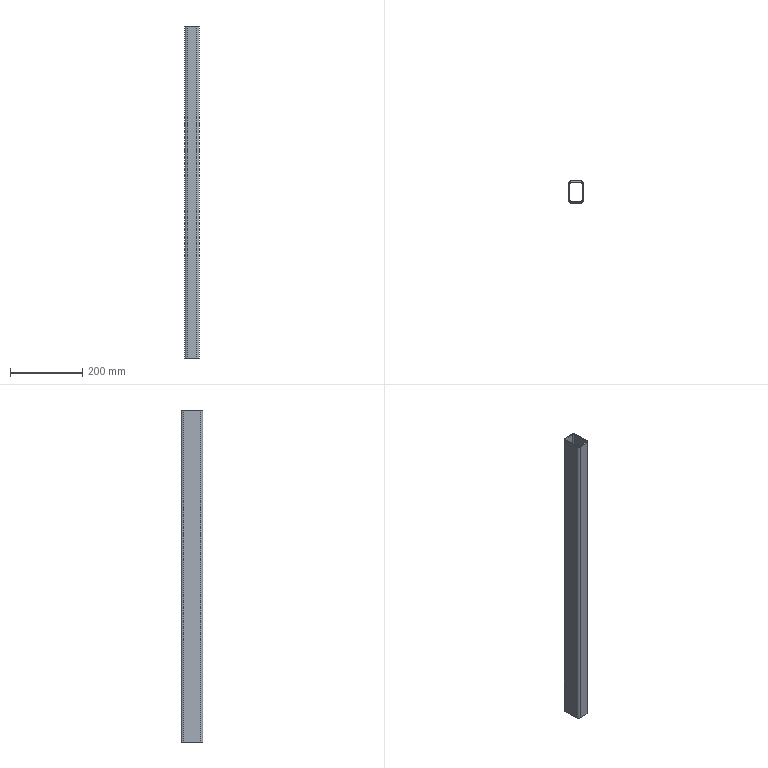Part | STEP file | Profile 4060920 | 1 solid | 18 faces | box 40 x 60 x 920 mm | volume 526856 mm3 | plane 10 | cylinder 8 | commonest cylinder face diameters 6.4 x4 12.8 x4
STEP:
#1=CARTESIAN_POINT('',(40.,6.4,-600.));
#2=VERTEX_POINT('',#1);
#3=CARTESIAN_POINT('',(40.,6.4,320.));
#4=VERTEX_POINT('',#3);
#5=CARTESIAN_POINT('',(40.,6.4,600.));
#6=DIRECTION('',(0.,0.,1.));
#7=VECTOR('',#6,1000.);
#8=LINE('',#5,#7);
#9=EDGE_CURVE('',#2,#4,#8,.T.);
#10=ORIENTED_EDGE('',*,*,#9,.F.);
#11=CARTESIAN_POINT('',(40.,53.6,-600.));
#12=VERTEX_POINT('',#11);
#13=CARTESIAN_POINT('',(40.,53.6,-600.));
#14=DIRECTION('',(0.,-1.,0.));
#15=VECTOR('',#14,1000.);
#16=LINE('',#13,#15);
#17=EDGE_CURVE('',#12,#2,#16,.T.);
#18=ORIENTED_EDGE('',*,*,#17,.F.);
#19=CARTESIAN_POINT('',(40.,53.6,320.));
#20=VERTEX_POINT('',#19);
#21=CARTESIAN_POINT('',(40.,53.6,600.));
#22=DIRECTION('',(0.,0.,-1.));
#23=VECTOR('',#22,1000.);
#24=LINE('',#21,#23);
#25=EDGE_CURVE('',#20,#12,#24,.T.);
#26=ORIENTED_EDGE('',*,*,#25,.F.);
#27=CARTESIAN_POINT('',(40.,53.6,320.));
#28=DIRECTION('',(0.,1.,0.));
#29=VECTOR('',#28,1000.);
#30=LINE('',#27,#29);
#31=EDGE_CURVE('',#4,#20,#30,.T.);
#32=ORIENTED_EDGE('',*,*,#31,.F.);
#33=EDGE_LOOP('',(#10,#18,#26,#32));
#34=FACE_OUTER_BOUND('',#33,.T.);
#35=CARTESIAN_POINT('',(40.,53.6,600.));
#36=DIRECTION('',(-1.,0.,0.));
#37=DIRECTION('',(0.,0.,1.));
#38=AXIS2_PLACEMENT_3D('',#35,#36,#37);
#39=PLANE('',#38);
#40=ADVANCED_FACE('',(#34),#39,.F.);
#41=CARTESIAN_POINT('',(0.,6.4,320.));
#42=VERTEX_POINT('',#41);
#43=CARTESIAN_POINT('',(6.4,0.,320.));
#44=VERTEX_POINT('',#43);
#45=CARTESIAN_POINT('',(6.4,6.4,320.));
#46=DIRECTION('',(0.,0.,1.));
#47=DIRECTION('',(-1.,0.,0.));
#48=AXIS2_PLACEMENT_3D('',#45,#46,#47);
#49=CIRCLE('',#48,6.4);
#50=EDGE_CURVE('',#42,#44,#49,.T.);
#51=ORIENTED_EDGE('',*,*,#50,.T.);
#52=CARTESIAN_POINT('',(33.6,0.,320.));
#53=VERTEX_POINT('',#52);
#54=CARTESIAN_POINT('',(33.6,0.,320.));
#55=DIRECTION('',(1.,0.,0.));
#56=VECTOR('',#55,1000.);
#57=LINE('',#54,#56);
#58=EDGE_CURVE('',#44,#53,#57,.T.);
#59=ORIENTED_EDGE('',*,*,#58,.T.);
#60=CARTESIAN_POINT('',(33.6,6.4,320.));
#61=DIRECTION('',(0.,0.,1.));
#62=DIRECTION('',(-1.,0.,0.));
#63=AXIS2_PLACEMENT_3D('',#60,#61,#62);
#64=CIRCLE('',#63,6.4);
#65=EDGE_CURVE('',#53,#4,#64,.T.);
#66=ORIENTED_EDGE('',*,*,#65,.T.);
#67=ORIENTED_EDGE('',*,*,#31,.T.);
#68=CARTESIAN_POINT('',(33.6,60.,320.));
#69=VERTEX_POINT('',#68);
#70=CARTESIAN_POINT('',(33.6,53.6,320.));
#71=DIRECTION('',(0.,0.,1.));
#72=DIRECTION('',(-1.,0.,0.));
#73=AXIS2_PLACEMENT_3D('',#70,#71,#72);
#74=CIRCLE('',#73,6.4);
#75=EDGE_CURVE('',#20,#69,#74,.T.);
#76=ORIENTED_EDGE('',*,*,#75,.T.);
#77=CARTESIAN_POINT('',(6.4,60.,320.));
#78=VERTEX_POINT('',#77);
#79=CARTESIAN_POINT('',(33.6,60.,320.));
#80=DIRECTION('',(-1.,0.,0.));
#81=VECTOR('',#80,1000.);
#82=LINE('',#79,#81);
#83=EDGE_CURVE('',#69,#78,#82,.T.);
#84=ORIENTED_EDGE('',*,*,#83,.T.);
#85=CARTESIAN_POINT('',(0.,53.6,320.));
#86=VERTEX_POINT('',#85);
#87=CARTESIAN_POINT('',(6.4,53.6,320.));
#88=DIRECTION('',(0.,0.,1.));
#89=DIRECTION('',(-1.,0.,0.));
#90=AXIS2_PLACEMENT_3D('',#87,#88,#89);
#91=CIRCLE('',#90,6.4);
#92=EDGE_CURVE('',#78,#86,#91,.T.);
#93=ORIENTED_EDGE('',*,*,#92,.T.);
#94=CARTESIAN_POINT('',(0.,6.4,320.));
#95=DIRECTION('',(0.,-1.,0.));
#96=VECTOR('',#95,1000.);
#97=LINE('',#94,#96);
#98=EDGE_CURVE('',#86,#42,#97,.T.);
#99=ORIENTED_EDGE('',*,*,#98,.T.);
#100=EDGE_LOOP('',(#51,#59,#66,#67,#76,#84,#93,#99));
#101=FACE_OUTER_BOUND('',#100,.T.);
#102=CARTESIAN_POINT('',(36.8,53.6,320.));
#103=VERTEX_POINT('',#102);
#104=CARTESIAN_POINT('',(36.8,6.4,320.));
#105=VERTEX_POINT('',#104);
#106=CARTESIAN_POINT('',(36.8,6.4,320.));
#107=DIRECTION('',(0.,-1.,0.));
#108=VECTOR('',#107,1000.);
#109=LINE('',#106,#108);
#110=EDGE_CURVE('',#103,#105,#109,.T.);
#111=ORIENTED_EDGE('',*,*,#110,.T.);
#112=CARTESIAN_POINT('',(33.6,3.2,320.));
#113=VERTEX_POINT('',#112);
#114=CARTESIAN_POINT('',(33.6,6.4,320.));
#115=DIRECTION('',(0.,0.,-1.));
#116=DIRECTION('',(-1.,0.,0.));
#117=AXIS2_PLACEMENT_3D('',#114,#115,#116);
#118=CIRCLE('',#117,3.2);
#119=EDGE_CURVE('',#105,#113,#118,.T.);
#120=ORIENTED_EDGE('',*,*,#119,.T.);
#121=CARTESIAN_POINT('',(6.4,3.2,320.));
#122=VERTEX_POINT('',#121);
#123=CARTESIAN_POINT('',(33.6,3.2,320.));
#124=DIRECTION('',(-1.,0.,0.));
#125=VECTOR('',#124,1000.);
#126=LINE('',#123,#125);
#127=EDGE_CURVE('',#113,#122,#126,.T.);
#128=ORIENTED_EDGE('',*,*,#127,.T.);
#129=CARTESIAN_POINT('',(3.2,6.4,320.));
#130=VERTEX_POINT('',#129);
#131=CARTESIAN_POINT('',(6.4,6.4,320.));
#132=DIRECTION('',(0.,0.,-1.));
#133=DIRECTION('',(-1.,0.,0.));
#134=AXIS2_PLACEMENT_3D('',#131,#132,#133);
#135=CIRCLE('',#134,3.2);
#136=EDGE_CURVE('',#122,#130,#135,.T.);
#137=ORIENTED_EDGE('',*,*,#136,.T.);
#138=CARTESIAN_POINT('',(3.2,53.6,320.));
#139=VERTEX_POINT('',#138);
#140=CARTESIAN_POINT('',(3.2,6.4,320.));
#141=DIRECTION('',(0.,1.,0.));
#142=VECTOR('',#141,1000.);
#143=LINE('',#140,#142);
#144=EDGE_CURVE('',#130,#139,#143,.T.);
#145=ORIENTED_EDGE('',*,*,#144,.T.);
#146=CARTESIAN_POINT('',(6.4,56.8,320.));
#147=VERTEX_POINT('',#146);
#148=CARTESIAN_POINT('',(6.4,53.6,320.));
#149=DIRECTION('',(0.,0.,-1.));
#150=DIRECTION('',(-1.,0.,0.));
#151=AXIS2_PLACEMENT_3D('',#148,#149,#150);
#152=CIRCLE('',#151,3.2);
#153=EDGE_CURVE('',#139,#147,#152,.T.);
#154=ORIENTED_EDGE('',*,*,#153,.T.);
#155=CARTESIAN_POINT('',(33.6,56.8,320.));
#156=VERTEX_POINT('',#155);
#157=CARTESIAN_POINT('',(33.6,56.8,320.));
#158=DIRECTION('',(1.,0.,0.));
#159=VECTOR('',#158,1000.);
#160=LINE('',#157,#159);
#161=EDGE_CURVE('',#147,#156,#160,.T.);
#162=ORIENTED_EDGE('',*,*,#161,.T.);
#163=CARTESIAN_POINT('',(33.6,53.6,320.));
#164=DIRECTION('',(0.,0.,-1.));
#165=DIRECTION('',(-1.,0.,0.));
#166=AXIS2_PLACEMENT_3D('',#163,#164,#165);
#167=CIRCLE('',#166,3.2);
#168=EDGE_CURVE('',#156,#103,#167,.T.);
#169=ORIENTED_EDGE('',*,*,#168,.T.);
#170=EDGE_LOOP('',(#111,#120,#128,#137,#145,#154,#162,#169));
#171=FACE_BOUND('',#170,.T.);
#172=CARTESIAN_POINT('',(33.6,6.4,320.));
#173=DIRECTION('',(0.,0.,1.));
#174=DIRECTION('',(1.,0.,0.));
#175=AXIS2_PLACEMENT_3D('',#172,#173,#174);
#176=PLANE('',#175);
#177=ADVANCED_FACE('',(#101,#171),#176,.T.);
#178=CARTESIAN_POINT('',(33.6,0.,-600.));
#179=VERTEX_POINT('',#178);
#180=CARTESIAN_POINT('',(33.6,0.,600.));
#181=DIRECTION('',(0.,0.,-1.));
#182=VECTOR('',#181,1000.);
#183=LINE('',#180,#182);
#184=EDGE_CURVE('',#53,#179,#183,.T.);
#185=ORIENTED_EDGE('',*,*,#184,.T.);
#186=CARTESIAN_POINT('',(33.6,6.4,-600.));
#187=DIRECTION('',(0.,0.,1.));
#188=DIRECTION('',(-1.,0.,0.));
#189=AXIS2_PLACEMENT_3D('',#186,#187,#188);
#190=CIRCLE('',#189,6.4);
#191=EDGE_CURVE('',#179,#2,#190,.T.);
#192=ORIENTED_EDGE('',*,*,#191,.T.);
#193=ORIENTED_EDGE('',*,*,#9,.T.);
#194=ORIENTED_EDGE('',*,*,#65,.F.);
#195=EDGE_LOOP('',(#185,#192,#193,#194));
#196=FACE_OUTER_BOUND('',#195,.T.);
#197=CARTESIAN_POINT('',(33.6,6.4,600.));
#198=DIRECTION('',(0.,0.,-1.));
#199=DIRECTION('',(-1.,0.,0.));
#200=AXIS2_PLACEMENT_3D('',#197,#198,#199);
#201=CYLINDRICAL_SURFACE('',#200,6.4);
#202=ADVANCED_FACE('',(#196),#201,.T.);
#203=ORIENTED_EDGE('',*,*,#191,.F.);
#204=CARTESIAN_POINT('',(6.4,0.,-600.));
#205=VERTEX_POINT('',#204);
#206=CARTESIAN_POINT('',(33.6,0.,-600.));
#207=DIRECTION('',(1.,0.,0.));
#208=VECTOR('',#207,1000.);
#209=LINE('',#206,#208);
#210=EDGE_CURVE('',#205,#179,#209,.T.);
#211=ORIENTED_EDGE('',*,*,#210,.F.);
#212=CARTESIAN_POINT('',(0.,6.4,-600.));
#213=VERTEX_POINT('',#212);
#214=CARTESIAN_POINT('',(6.4,6.4,-600.));
#215=DIRECTION('',(0.,0.,1.));
#216=DIRECTION('',(-1.,0.,0.));
#217=AXIS2_PLACEMENT_3D('',#214,#215,#216);
#218=CIRCLE('',#217,6.4);
#219=EDGE_CURVE('',#213,#205,#218,.T.);
#220=ORIENTED_EDGE('',*,*,#219,.F.);
#221=CARTESIAN_POINT('',(0.,53.6,-600.));
#222=VERTEX_POINT('',#221);
#223=CARTESIAN_POINT('',(0.,53.6,-600.));
#224=DIRECTION('',(0.,-1.,0.));
#225=VECTOR('',#224,1000.);
#226=LINE('',#223,#225);
#227=EDGE_CURVE('',#222,#213,#226,.T.);
#228=ORIENTED_EDGE('',*,*,#227,.F.);
#229=CARTESIAN_POINT('',(6.4,60.,-600.));
#230=VERTEX_POINT('',#229);
#231=CARTESIAN_POINT('',(6.4,53.6,-600.));
#232=DIRECTION('',(0.,0.,1.));
#233=DIRECTION('',(-1.,0.,0.));
#234=AXIS2_PLACEMENT_3D('',#231,#232,#233);
#235=CIRCLE('',#234,6.4);
#236=EDGE_CURVE('',#230,#222,#235,.T.);
#237=ORIENTED_EDGE('',*,*,#236,.F.);
#238=CARTESIAN_POINT('',(33.6,60.,-600.));
#239=VERTEX_POINT('',#238);
#240=CARTESIAN_POINT('',(33.6,60.,-600.));
#241=DIRECTION('',(-1.,0.,0.));
#242=VECTOR('',#241,1000.);
#243=LINE('',#240,#242);
#244=EDGE_CURVE('',#239,#230,#243,.T.);
#245=ORIENTED_EDGE('',*,*,#244,.F.);
#246=CARTESIAN_POINT('',(33.6,53.6,-600.));
#247=DIRECTION('',(0.,0.,1.));
#248=DIRECTION('',(-1.,0.,0.));
#249=AXIS2_PLACEMENT_3D('',#246,#247,#248);
#250=CIRCLE('',#249,6.4);
#251=EDGE_CURVE('',#12,#239,#250,.T.);
#252=ORIENTED_EDGE('',*,*,#251,.F.);
#253=ORIENTED_EDGE('',*,*,#17,.T.);
#254=EDGE_LOOP('',(#203,#211,#220,#228,#237,#245,#252,#253));
#255=FACE_OUTER_BOUND('',#254,.T.);
#256=CARTESIAN_POINT('',(6.4,3.2,-600.));
#257=VERTEX_POINT('',#256);
#258=CARTESIAN_POINT('',(3.2,6.4,-600.));
#259=VERTEX_POINT('',#258);
#260=CARTESIAN_POINT('',(6.4,6.4,-600.));
#261=DIRECTION('',(0.,0.,-1.));
#262=DIRECTION('',(-1.,0.,0.));
#263=AXIS2_PLACEMENT_3D('',#260,#261,#262);
#264=CIRCLE('',#263,3.2);
#265=EDGE_CURVE('',#257,#259,#264,.T.);
#266=ORIENTED_EDGE('',*,*,#265,.F.);
#267=CARTESIAN_POINT('',(33.6,3.2,-600.));
#268=VERTEX_POINT('',#267);
#269=CARTESIAN_POINT('',(33.6,3.2,-600.));
#270=DIRECTION('',(-1.,0.,0.));
#271=VECTOR('',#270,1000.);
#272=LINE('',#269,#271);
#273=EDGE_CURVE('',#268,#257,#272,.T.);
#274=ORIENTED_EDGE('',*,*,#273,.F.);
#275=CARTESIAN_POINT('',(36.8,6.4,-600.));
#276=VERTEX_POINT('',#275);
#277=CARTESIAN_POINT('',(33.6,6.4,-600.));
#278=DIRECTION('',(0.,0.,-1.));
#279=DIRECTION('',(-1.,0.,0.));
#280=AXIS2_PLACEMENT_3D('',#277,#278,#279);
#281=CIRCLE('',#280,3.2);
#282=EDGE_CURVE('',#276,#268,#281,.T.);
#283=ORIENTED_EDGE('',*,*,#282,.F.);
#284=CARTESIAN_POINT('',(36.8,53.6,-600.));
#285=VERTEX_POINT('',#284);
#286=CARTESIAN_POINT('',(36.8,53.6,-600.));
#287=DIRECTION('',(0.,-1.,0.));
#288=VECTOR('',#287,1000.);
#289=LINE('',#286,#288);
#290=EDGE_CURVE('',#285,#276,#289,.T.);
#291=ORIENTED_EDGE('',*,*,#290,.F.);
#292=CARTESIAN_POINT('',(33.6,56.8,-600.));
#293=VERTEX_POINT('',#292);
#294=CARTESIAN_POINT('',(33.6,53.6,-600.));
#295=DIRECTION('',(0.,0.,-1.));
#296=DIRECTION('',(-1.,0.,0.));
#297=AXIS2_PLACEMENT_3D('',#294,#295,#296);
#298=CIRCLE('',#297,3.2);
#299=EDGE_CURVE('',#293,#285,#298,.T.);
#300=ORIENTED_EDGE('',*,*,#299,.F.);
#301=CARTESIAN_POINT('',(6.4,56.8,-600.));
#302=VERTEX_POINT('',#301);
#303=CARTESIAN_POINT('',(33.6,56.8,-600.));
#304=DIRECTION('',(1.,0.,0.));
#305=VECTOR('',#304,1000.);
#306=LINE('',#303,#305);
#307=EDGE_CURVE('',#302,#293,#306,.T.);
#308=ORIENTED_EDGE('',*,*,#307,.F.);
#309=CARTESIAN_POINT('',(3.2,53.6,-600.));
#310=VERTEX_POINT('',#309);
#311=CARTESIAN_POINT('',(6.4,53.6,-600.));
#312=DIRECTION('',(0.,0.,-1.));
#313=DIRECTION('',(-1.,0.,0.));
#314=AXIS2_PLACEMENT_3D('',#311,#312,#313);
#315=CIRCLE('',#314,3.2);
#316=EDGE_CURVE('',#310,#302,#315,.T.);
#317=ORIENTED_EDGE('',*,*,#316,.F.);
#318=CARTESIAN_POINT('',(3.2,53.6,-600.));
#319=DIRECTION('',(0.,1.,0.));
#320=VECTOR('',#319,1000.);
#321=LINE('',#318,#320);
#322=EDGE_CURVE('',#259,#310,#321,.T.);
#323=ORIENTED_EDGE('',*,*,#322,.F.);
#324=EDGE_LOOP('',(#266,#274,#283,#291,#300,#308,#317,#323));
#325=FACE_BOUND('',#324,.T.);
#326=CARTESIAN_POINT('',(33.6,53.6,-600.));
#327=DIRECTION('',(0.,0.,1.));
#328=DIRECTION('',(1.,0.,0.));
#329=AXIS2_PLACEMENT_3D('',#326,#327,#328);
#330=PLANE('',#329);
#331=ADVANCED_FACE('',(#255,#325),#330,.F.);
#332=ORIENTED_EDGE('',*,*,#25,.T.);
#333=ORIENTED_EDGE('',*,*,#251,.T.);
#334=CARTESIAN_POINT('',(33.6,60.,600.));
#335=DIRECTION('',(0.,0.,1.));
#336=VECTOR('',#335,1000.);
#337=LINE('',#334,#336);
#338=EDGE_CURVE('',#239,#69,#337,.T.);
#339=ORIENTED_EDGE('',*,*,#338,.T.);
#340=ORIENTED_EDGE('',*,*,#75,.F.);
#341=EDGE_LOOP('',(#332,#333,#339,#340));
#342=FACE_OUTER_BOUND('',#341,.T.);
#343=CARTESIAN_POINT('',(33.6,53.6,600.));
#344=DIRECTION('',(0.,0.,-1.));
#345=DIRECTION('',(-1.,0.,0.));
#346=AXIS2_PLACEMENT_3D('',#343,#344,#345);
#347=CYLINDRICAL_SURFACE('',#346,6.4);
#348=ADVANCED_FACE('',(#342),#347,.T.);
#349=CARTESIAN_POINT('',(6.4,0.,600.));
#350=DIRECTION('',(0.,0.,1.));
#351=VECTOR('',#350,1000.);
#352=LINE('',#349,#351);
#353=EDGE_CURVE('',#205,#44,#352,.T.);
#354=ORIENTED_EDGE('',*,*,#353,.F.);
#355=ORIENTED_EDGE('',*,*,#210,.T.);
#356=ORIENTED_EDGE('',*,*,#184,.F.);
#357=ORIENTED_EDGE('',*,*,#58,.F.);
#358=EDGE_LOOP('',(#354,#355,#356,#357));
#359=FACE_OUTER_BOUND('',#358,.T.);
#360=CARTESIAN_POINT('',(6.4,0.,600.));
#361=DIRECTION('',(0.,1.,0.));
#362=DIRECTION('',(-1.,0.,0.));
#363=AXIS2_PLACEMENT_3D('',#360,#361,#362);
#364=PLANE('',#363);
#365=ADVANCED_FACE('',(#359),#364,.F.);
#366=CARTESIAN_POINT('',(0.,6.4,600.));
#367=DIRECTION('',(0.,0.,-1.));
#368=VECTOR('',#367,1000.);
#369=LINE('',#366,#368);
#370=EDGE_CURVE('',#42,#213,#369,.T.);
#371=ORIENTED_EDGE('',*,*,#370,.T.);
#372=ORIENTED_EDGE('',*,*,#219,.T.);
#373=ORIENTED_EDGE('',*,*,#353,.T.);
#374=ORIENTED_EDGE('',*,*,#50,.F.);
#375=EDGE_LOOP('',(#371,#372,#373,#374));
#376=FACE_OUTER_BOUND('',#375,.T.);
#377=CARTESIAN_POINT('',(6.4,6.4,600.));
#378=DIRECTION('',(0.,0.,-1.));
#379=DIRECTION('',(-1.,0.,0.));
#380=AXIS2_PLACEMENT_3D('',#377,#378,#379);
#381=CYLINDRICAL_SURFACE('',#380,6.4);
#382=ADVANCED_FACE('',(#376),#381,.T.);
#383=CARTESIAN_POINT('',(0.,53.6,600.));
#384=DIRECTION('',(0.,0.,1.));
#385=VECTOR('',#384,1000.);
#386=LINE('',#383,#385);
#387=EDGE_CURVE('',#222,#86,#386,.T.);
#388=ORIENTED_EDGE('',*,*,#387,.F.);
#389=ORIENTED_EDGE('',*,*,#227,.T.);
#390=ORIENTED_EDGE('',*,*,#370,.F.);
#391=ORIENTED_EDGE('',*,*,#98,.F.);
#392=EDGE_LOOP('',(#388,#389,#390,#391));
#393=FACE_OUTER_BOUND('',#392,.T.);
#394=CARTESIAN_POINT('',(0.,6.4,600.));
#395=DIRECTION('',(1.,0.,0.));
#396=DIRECTION('',(0.,1.,0.));
#397=AXIS2_PLACEMENT_3D('',#394,#395,#396);
#398=PLANE('',#397);
#399=ADVANCED_FACE('',(#393),#398,.F.);
#400=CARTESIAN_POINT('',(6.4,60.,600.));
#401=DIRECTION('',(0.,0.,-1.));
#402=VECTOR('',#401,1000.);
#403=LINE('',#400,#402);
#404=EDGE_CURVE('',#78,#230,#403,.T.);
#405=ORIENTED_EDGE('',*,*,#404,.T.);
#406=ORIENTED_EDGE('',*,*,#236,.T.);
#407=ORIENTED_EDGE('',*,*,#387,.T.);
#408=ORIENTED_EDGE('',*,*,#92,.F.);
#409=EDGE_LOOP('',(#405,#406,#407,#408));
#410=FACE_OUTER_BOUND('',#409,.T.);
#411=CARTESIAN_POINT('',(6.4,53.6,600.));
#412=DIRECTION('',(0.,0.,-1.));
#413=DIRECTION('',(-1.,0.,0.));
#414=AXIS2_PLACEMENT_3D('',#411,#412,#413);
#415=CYLINDRICAL_SURFACE('',#414,6.4);
#416=ADVANCED_FACE('',(#410),#415,.T.);
#417=ORIENTED_EDGE('',*,*,#338,.F.);
#418=ORIENTED_EDGE('',*,*,#244,.T.);
#419=ORIENTED_EDGE('',*,*,#404,.F.);
#420=ORIENTED_EDGE('',*,*,#83,.F.);
#421=EDGE_LOOP('',(#417,#418,#419,#420));
#422=FACE_OUTER_BOUND('',#421,.T.);
#423=CARTESIAN_POINT('',(33.6,60.,600.));
#424=DIRECTION('',(0.,-1.,0.));
#425=DIRECTION('',(0.,0.,-1.));
#426=AXIS2_PLACEMENT_3D('',#423,#424,#425);
#427=PLANE('',#426);
#428=ADVANCED_FACE('',(#422),#427,.F.);
#429=CARTESIAN_POINT('',(36.8,6.4,600.));
#430=DIRECTION('',(0.,0.,1.));
#431=VECTOR('',#430,1000.);
#432=LINE('',#429,#431);
#433=EDGE_CURVE('',#276,#105,#432,.T.);
#434=ORIENTED_EDGE('',*,*,#433,.F.);
#435=ORIENTED_EDGE('',*,*,#282,.T.);
#436=CARTESIAN_POINT('',(33.6,3.2,600.));
#437=DIRECTION('',(0.,0.,-1.));
#438=VECTOR('',#437,1000.);
#439=LINE('',#436,#438);
#440=EDGE_CURVE('',#113,#268,#439,.T.);
#441=ORIENTED_EDGE('',*,*,#440,.F.);
#442=ORIENTED_EDGE('',*,*,#119,.F.);
#443=EDGE_LOOP('',(#434,#435,#441,#442));
#444=FACE_OUTER_BOUND('',#443,.T.);
#445=CARTESIAN_POINT('',(33.6,6.4,600.));
#446=DIRECTION('',(0.,0.,-1.));
#447=DIRECTION('',(-1.,0.,0.));
#448=AXIS2_PLACEMENT_3D('',#445,#446,#447);
#449=CYLINDRICAL_SURFACE('',#448,3.2);
#450=ADVANCED_FACE('',(#444),#449,.F.);
#451=CARTESIAN_POINT('',(36.8,53.6,600.));
#452=DIRECTION('',(0.,0.,-1.));
#453=VECTOR('',#452,1000.);
#454=LINE('',#451,#453);
#455=EDGE_CURVE('',#103,#285,#454,.T.);
#456=ORIENTED_EDGE('',*,*,#455,.T.);
#457=ORIENTED_EDGE('',*,*,#290,.T.);
#458=ORIENTED_EDGE('',*,*,#433,.T.);
#459=ORIENTED_EDGE('',*,*,#110,.F.);
#460=EDGE_LOOP('',(#456,#457,#458,#459));
#461=FACE_OUTER_BOUND('',#460,.T.);
#462=CARTESIAN_POINT('',(36.8,53.6,600.));
#463=DIRECTION('',(-1.,0.,0.));
#464=DIRECTION('',(0.,0.,1.));
#465=AXIS2_PLACEMENT_3D('',#462,#463,#464);
#466=PLANE('',#465);
#467=ADVANCED_FACE('',(#461),#466,.T.);
#468=CARTESIAN_POINT('',(33.6,56.8,600.));
#469=DIRECTION('',(0.,0.,1.));
#470=VECTOR('',#469,1000.);
#471=LINE('',#468,#470);
#472=EDGE_CURVE('',#293,#156,#471,.T.);
#473=ORIENTED_EDGE('',*,*,#472,.F.);
#474=ORIENTED_EDGE('',*,*,#299,.T.);
#475=ORIENTED_EDGE('',*,*,#455,.F.);
#476=ORIENTED_EDGE('',*,*,#168,.F.);
#477=EDGE_LOOP('',(#473,#474,#475,#476));
#478=FACE_OUTER_BOUND('',#477,.T.);
#479=CARTESIAN_POINT('',(33.6,53.6,600.));
#480=DIRECTION('',(0.,0.,-1.));
#481=DIRECTION('',(-1.,0.,0.));
#482=AXIS2_PLACEMENT_3D('',#479,#480,#481);
#483=CYLINDRICAL_SURFACE('',#482,3.2);
#484=ADVANCED_FACE('',(#478),#483,.F.);
#485=CARTESIAN_POINT('',(6.4,56.8,600.));
#486=DIRECTION('',(0.,0.,-1.));
#487=VECTOR('',#486,1000.);
#488=LINE('',#485,#487);
#489=EDGE_CURVE('',#147,#302,#488,.T.);
#490=ORIENTED_EDGE('',*,*,#489,.T.);
#491=ORIENTED_EDGE('',*,*,#307,.T.);
#492=ORIENTED_EDGE('',*,*,#472,.T.);
#493=ORIENTED_EDGE('',*,*,#161,.F.);
#494=EDGE_LOOP('',(#490,#491,#492,#493));
#495=FACE_OUTER_BOUND('',#494,.T.);
#496=CARTESIAN_POINT('',(33.6,56.8,600.));
#497=DIRECTION('',(0.,-1.,0.));
#498=DIRECTION('',(0.,0.,-1.));
#499=AXIS2_PLACEMENT_3D('',#496,#497,#498);
#500=PLANE('',#499);
#501=ADVANCED_FACE('',(#495),#500,.T.);
#502=CARTESIAN_POINT('',(3.2,53.6,600.));
#503=DIRECTION('',(0.,0.,1.));
#504=VECTOR('',#503,1000.);
#505=LINE('',#502,#504);
#506=EDGE_CURVE('',#310,#139,#505,.T.);
#507=ORIENTED_EDGE('',*,*,#506,.F.);
#508=ORIENTED_EDGE('',*,*,#316,.T.);
#509=ORIENTED_EDGE('',*,*,#489,.F.);
#510=ORIENTED_EDGE('',*,*,#153,.F.);
#511=EDGE_LOOP('',(#507,#508,#509,#510));
#512=FACE_OUTER_BOUND('',#511,.T.);
#513=CARTESIAN_POINT('',(6.4,53.6,600.));
#514=DIRECTION('',(0.,0.,-1.));
#515=DIRECTION('',(-1.,0.,0.));
#516=AXIS2_PLACEMENT_3D('',#513,#514,#515);
#517=CYLINDRICAL_SURFACE('',#516,3.2);
#518=ADVANCED_FACE('',(#512),#517,.F.);
#519=CARTESIAN_POINT('',(3.2,6.4,600.));
#520=DIRECTION('',(0.,0.,-1.));
#521=VECTOR('',#520,1000.);
#522=LINE('',#519,#521);
#523=EDGE_CURVE('',#130,#259,#522,.T.);
#524=ORIENTED_EDGE('',*,*,#523,.T.);
#525=ORIENTED_EDGE('',*,*,#322,.T.);
#526=ORIENTED_EDGE('',*,*,#506,.T.);
#527=ORIENTED_EDGE('',*,*,#144,.F.);
#528=EDGE_LOOP('',(#524,#525,#526,#527));
#529=FACE_OUTER_BOUND('',#528,.T.);
#530=CARTESIAN_POINT('',(3.2,6.4,600.));
#531=DIRECTION('',(1.,0.,0.));
#532=DIRECTION('',(0.,1.,0.));
#533=AXIS2_PLACEMENT_3D('',#530,#531,#532);
#534=PLANE('',#533);
#535=ADVANCED_FACE('',(#529),#534,.T.);
#536=CARTESIAN_POINT('',(6.4,3.2,600.));
#537=DIRECTION('',(0.,0.,1.));
#538=VECTOR('',#537,1000.);
#539=LINE('',#536,#538);
#540=EDGE_CURVE('',#257,#122,#539,.T.);
#541=ORIENTED_EDGE('',*,*,#540,.F.);
#542=ORIENTED_EDGE('',*,*,#265,.T.);
#543=ORIENTED_EDGE('',*,*,#523,.F.);
#544=ORIENTED_EDGE('',*,*,#136,.F.);
#545=EDGE_LOOP('',(#541,#542,#543,#544));
#546=FACE_OUTER_BOUND('',#545,.T.);
#547=CARTESIAN_POINT('',(6.4,6.4,600.));
#548=DIRECTION('',(0.,0.,-1.));
#549=DIRECTION('',(-1.,0.,0.));
#550=AXIS2_PLACEMENT_3D('',#547,#548,#549);
#551=CYLINDRICAL_SURFACE('',#550,3.2);
#552=ADVANCED_FACE('',(#546),#551,.F.);
#553=ORIENTED_EDGE('',*,*,#440,.T.);
#554=ORIENTED_EDGE('',*,*,#273,.T.);
#555=ORIENTED_EDGE('',*,*,#540,.T.);
#556=ORIENTED_EDGE('',*,*,#127,.F.);
#557=EDGE_LOOP('',(#553,#554,#555,#556));
#558=FACE_OUTER_BOUND('',#557,.T.);
#559=CARTESIAN_POINT('',(6.4,3.2,600.));
#560=DIRECTION('',(0.,1.,0.));
#561=DIRECTION('',(-1.,0.,0.));
#562=AXIS2_PLACEMENT_3D('',#559,#560,#561);
#563=PLANE('',#562);
#564=ADVANCED_FACE('',(#558),#563,.T.);
#565=CLOSED_SHELL('',(#40,#177,#202,#331,#348,#365,#382,#399,#416,#428,#450,#467,#484,#501,#518,#535,#552,#564));
#566=MANIFOLD_SOLID_BREP('',#565);
#567=CARTESIAN_POINT('',(0.,0.,0.));
#568=DIRECTION('',(0.,0.,1.));
#569=DIRECTION('',(1.,0.,0.));
#570=AXIS2_PLACEMENT_3D('',#567,#568,#569);
#571=(LENGTH_UNIT()NAMED_UNIT(*)SI_UNIT(.MILLI.,.METRE.));
#572=UNCERTAINTY_MEASURE_WITH_UNIT(LENGTH_MEASURE(0.00001),#571,'','');
#573=(NAMED_UNIT(*)PLANE_ANGLE_UNIT()SI_UNIT($,.RADIAN.));
#574=(NAMED_UNIT(*)SI_UNIT($,.STERADIAN.)SOLID_ANGLE_UNIT());
#575=(GEOMETRIC_REPRESENTATION_CONTEXT(3)GLOBAL_UNCERTAINTY_ASSIGNED_CONTEXT((#572))GLOBAL_UNIT_ASSIGNED_CONTEXT((#571,#573,#574))REPRESENTATION_CONTEXT('',''));
#576=ADVANCED_BREP_SHAPE_REPRESENTATION('',(#566,#570),#575);